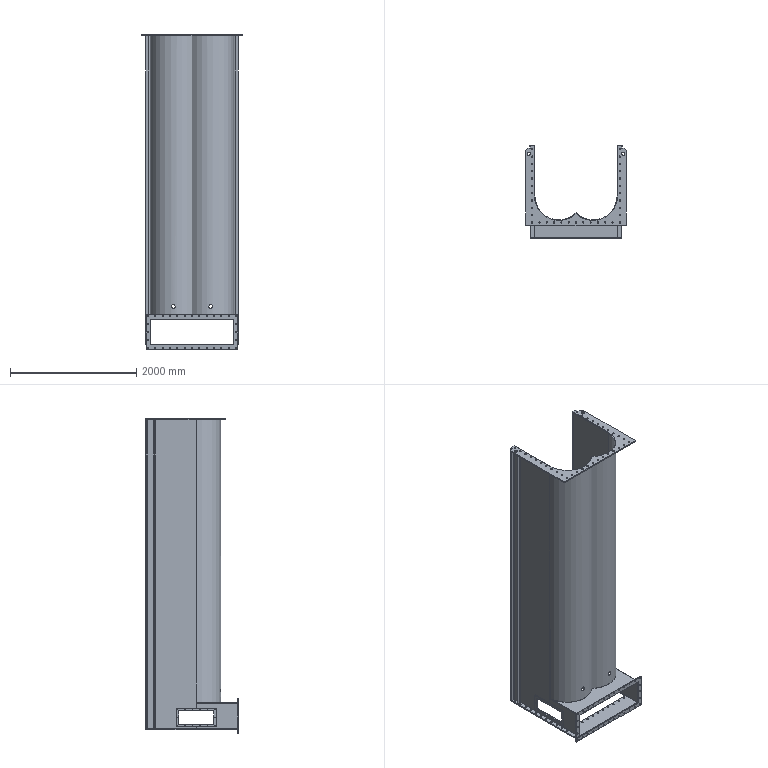Part | SolidWorks | features ICE 14, HoleWzd 6, MirrorPattern 6, LPattern 5, CombineBodies 3, MirrorSolid 3, MoveFace 3, Extrusion 1, MoveCopyBody 1, Split 1 | 11 solids | 426 faces | box 1600 x 1465 x 4987 mm | volume 200673004 mm3 | cylinder 306 | plane 120 | commonest cylinder face diameters 19.5 x132 8.5 x84 18 x64 778 x6 30 x4 48 x4